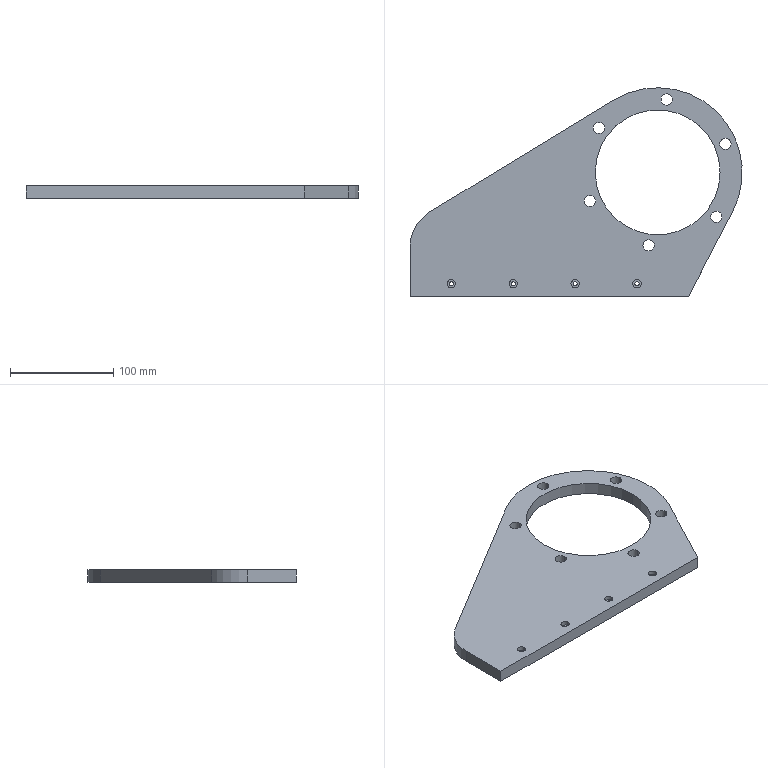Part | SolidWorks | features ICE 5, Extrusion 1 | 1 solid | 54 faces | box 322 x 202 x 12 mm | volume 411603 mm3 | cylinder 40 | plane 14 | commonest cylinder face diameters 8 x16 11 x12 4 x8 121 x2 80 x1 164 x1